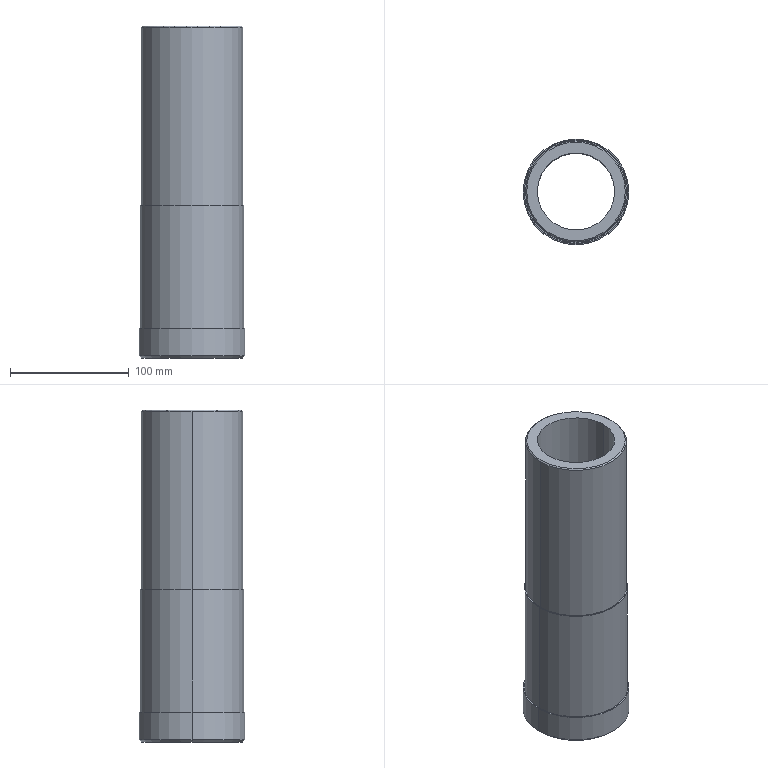Part | SolidWorks | features Chamfer 2, ICE 2, Extrusion 1 | 1 solid | 16 faces | box 89 x 89 x 279.1 mm | volume 698533 mm3 | cylinder 8 | cone 4 | plane 4 | commonest cylinder face diameters 65 x2 85 x2 87 x2 89 x2
STEP:
#1=CARTESIAN_POINT('',(41.5,0.,279.1));
#2=VERTEX_POINT('',#1);
#3=CARTESIAN_POINT('',(-41.5,0.,279.1));
#4=VERTEX_POINT('',#3);
#5=CARTESIAN_POINT('',(0.,0.,279.1));
#6=DIRECTION('',(0.,0.,1.));
#7=DIRECTION('',(1.,0.,0.));
#8=AXIS2_PLACEMENT_3D('',#5,#6,#7);
#9=CIRCLE('',#8,41.5);
#10=EDGE_CURVE('',#2,#4,#9,.T.);
#11=ORIENTED_EDGE('',*,*,#10,.F.);
#12=CARTESIAN_POINT('',(42.5,0.,278.1));
#13=VERTEX_POINT('',#12);
#14=CARTESIAN_POINT('',(41.5,0.,279.1));
#15=DIRECTION('',(0.7071,0.,-0.7071));
#16=VECTOR('',#15,1000.);
#17=LINE('',#14,#16);
#18=EDGE_CURVE('',#2,#13,#17,.T.);
#19=ORIENTED_EDGE('',*,*,#18,.T.);
#20=CARTESIAN_POINT('',(-42.5,0.,278.1));
#21=VERTEX_POINT('',#20);
#22=CARTESIAN_POINT('',(0.,0.,278.1));
#23=DIRECTION('',(0.,0.,-1.));
#24=DIRECTION('',(1.,0.,0.));
#25=AXIS2_PLACEMENT_3D('',#22,#23,#24);
#26=CIRCLE('',#25,42.5);
#27=EDGE_CURVE('',#21,#13,#26,.T.);
#28=ORIENTED_EDGE('',*,*,#27,.F.);
#29=CARTESIAN_POINT('',(-41.5,0.,279.1));
#30=DIRECTION('',(-0.7071,0.,-0.7071));
#31=VECTOR('',#30,1000.);
#32=LINE('',#29,#31);
#33=EDGE_CURVE('',#4,#21,#32,.T.);
#34=ORIENTED_EDGE('',*,*,#33,.F.);
#35=EDGE_LOOP('',(#11,#19,#28,#34));
#36=FACE_OUTER_BOUND('',#35,.T.);
#37=CARTESIAN_POINT('',(0.,0.,279.1));
#38=DIRECTION('',(0.,0.,-1.));
#39=DIRECTION('',(-1.,0.,0.));
#40=AXIS2_PLACEMENT_3D('',#37,#38,#39);
#41=CONICAL_SURFACE('',#40,41.5,0.7854);
#42=ADVANCED_FACE('',(#36),#41,.T.);
#43=CARTESIAN_POINT('',(-42.5,0.,0.));
#44=VERTEX_POINT('',#43);
#45=CARTESIAN_POINT('',(42.5,0.,0.));
#46=VERTEX_POINT('',#45);
#47=CARTESIAN_POINT('',(0.,0.,0.));
#48=DIRECTION('',(0.,0.,-1.));
#49=DIRECTION('',(1.,0.,0.));
#50=AXIS2_PLACEMENT_3D('',#47,#48,#49);
#51=CIRCLE('',#50,42.5);
#52=EDGE_CURVE('',#44,#46,#51,.T.);
#53=ORIENTED_EDGE('',*,*,#52,.F.);
#54=CARTESIAN_POINT('',(-44.5,0.,2.));
#55=VERTEX_POINT('',#54);
#56=CARTESIAN_POINT('',(-44.5,0.,2.));
#57=DIRECTION('',(-0.7071,0.,0.7071));
#58=VECTOR('',#57,1000.);
#59=LINE('',#56,#58);
#60=EDGE_CURVE('',#44,#55,#59,.T.);
#61=ORIENTED_EDGE('',*,*,#60,.T.);
#62=CARTESIAN_POINT('',(44.5,0.,2.));
#63=VERTEX_POINT('',#62);
#64=CARTESIAN_POINT('',(0.,0.,2.));
#65=DIRECTION('',(0.,0.,1.));
#66=DIRECTION('',(1.,0.,0.));
#67=AXIS2_PLACEMENT_3D('',#64,#65,#66);
#68=CIRCLE('',#67,44.5);
#69=EDGE_CURVE('',#63,#55,#68,.T.);
#70=ORIENTED_EDGE('',*,*,#69,.F.);
#71=CARTESIAN_POINT('',(44.5,0.,2.));
#72=DIRECTION('',(0.7071,0.,0.7071));
#73=VECTOR('',#72,1000.);
#74=LINE('',#71,#73);
#75=EDGE_CURVE('',#46,#63,#74,.T.);
#76=ORIENTED_EDGE('',*,*,#75,.F.);
#77=EDGE_LOOP('',(#53,#61,#70,#76));
#78=FACE_OUTER_BOUND('',#77,.T.);
#79=CARTESIAN_POINT('',(0.,0.,2.));
#80=DIRECTION('',(0.,0.,1.));
#81=DIRECTION('',(1.,0.,0.));
#82=AXIS2_PLACEMENT_3D('',#79,#80,#81);
#83=CONICAL_SURFACE('',#82,44.5,0.7854);
#84=ADVANCED_FACE('',(#78),#83,.T.);
#85=CARTESIAN_POINT('',(42.5,0.,128.4));
#86=VERTEX_POINT('',#85);
#87=CARTESIAN_POINT('',(-42.5,0.,128.4));
#88=VERTEX_POINT('',#87);
#89=CARTESIAN_POINT('',(0.,0.,128.4));
#90=DIRECTION('',(0.,0.,1.));
#91=DIRECTION('',(1.,0.,0.));
#92=AXIS2_PLACEMENT_3D('',#89,#90,#91);
#93=CIRCLE('',#92,42.5);
#94=EDGE_CURVE('',#86,#88,#93,.T.);
#95=ORIENTED_EDGE('',*,*,#94,.T.);
#96=CARTESIAN_POINT('',(-42.5,0.,128.4));
#97=DIRECTION('',(0.,0.,1.));
#98=VECTOR('',#97,1000.);
#99=LINE('',#96,#98);
#100=EDGE_CURVE('',#88,#21,#99,.T.);
#101=ORIENTED_EDGE('',*,*,#100,.T.);
#102=ORIENTED_EDGE('',*,*,#27,.T.);
#103=CARTESIAN_POINT('',(42.5,0.,128.4));
#104=DIRECTION('',(0.,0.,1.));
#105=VECTOR('',#104,1000.);
#106=LINE('',#103,#105);
#107=EDGE_CURVE('',#86,#13,#106,.T.);
#108=ORIENTED_EDGE('',*,*,#107,.F.);
#109=EDGE_LOOP('',(#95,#101,#102,#108));
#110=FACE_OUTER_BOUND('',#109,.T.);
#111=CARTESIAN_POINT('',(0.,0.,128.4));
#112=DIRECTION('',(0.,0.,1.));
#113=DIRECTION('',(1.,0.,0.));
#114=AXIS2_PLACEMENT_3D('',#111,#112,#113);
#115=CYLINDRICAL_SURFACE('',#114,42.5);
#116=ADVANCED_FACE('',(#110),#115,.T.);
#117=CARTESIAN_POINT('',(-32.5,0.,279.1));
#118=VERTEX_POINT('',#117);
#119=CARTESIAN_POINT('',(32.5,0.,279.1));
#120=VERTEX_POINT('',#119);
#121=CARTESIAN_POINT('',(0.,0.,279.1));
#122=DIRECTION('',(0.,0.,1.));
#123=DIRECTION('',(1.,0.,0.));
#124=AXIS2_PLACEMENT_3D('',#121,#122,#123);
#125=CIRCLE('',#124,32.5);
#126=EDGE_CURVE('',#118,#120,#125,.T.);
#127=ORIENTED_EDGE('',*,*,#126,.T.);
#128=CARTESIAN_POINT('',(32.5,0.,0.));
#129=VERTEX_POINT('',#128);
#130=CARTESIAN_POINT('',(32.5,0.,279.1));
#131=DIRECTION('',(0.,0.,-1.));
#132=VECTOR('',#131,1000.);
#133=LINE('',#130,#132);
#134=EDGE_CURVE('',#120,#129,#133,.T.);
#135=ORIENTED_EDGE('',*,*,#134,.T.);
#136=CARTESIAN_POINT('',(-32.5,0.,0.));
#137=VERTEX_POINT('',#136);
#138=CARTESIAN_POINT('',(0.,0.,0.));
#139=DIRECTION('',(0.,0.,1.));
#140=DIRECTION('',(1.,0.,0.));
#141=AXIS2_PLACEMENT_3D('',#138,#139,#140);
#142=CIRCLE('',#141,32.5);
#143=EDGE_CURVE('',#137,#129,#142,.T.);
#144=ORIENTED_EDGE('',*,*,#143,.F.);
#145=CARTESIAN_POINT('',(-32.5,0.,279.1));
#146=DIRECTION('',(0.,0.,-1.));
#147=VECTOR('',#146,1000.);
#148=LINE('',#145,#147);
#149=EDGE_CURVE('',#118,#137,#148,.T.);
#150=ORIENTED_EDGE('',*,*,#149,.F.);
#151=EDGE_LOOP('',(#127,#135,#144,#150));
#152=FACE_OUTER_BOUND('',#151,.T.);
#153=CARTESIAN_POINT('',(0.,0.,279.1));
#154=DIRECTION('',(0.,0.,-1.));
#155=DIRECTION('',(-1.,0.,0.));
#156=AXIS2_PLACEMENT_3D('',#153,#154,#155);
#157=CYLINDRICAL_SURFACE('',#156,32.5);
#158=ADVANCED_FACE('',(#152),#157,.F.);
#159=CARTESIAN_POINT('',(-44.5,0.,25.));
#160=VERTEX_POINT('',#159);
#161=CARTESIAN_POINT('',(44.5,0.,25.));
#162=VERTEX_POINT('',#161);
#163=CARTESIAN_POINT('',(0.,0.,25.));
#164=DIRECTION('',(0.,0.,-1.));
#165=DIRECTION('',(-1.,0.,0.));
#166=AXIS2_PLACEMENT_3D('',#163,#164,#165);
#167=CIRCLE('',#166,44.5);
#168=EDGE_CURVE('',#160,#162,#167,.T.);
#169=ORIENTED_EDGE('',*,*,#168,.T.);
#170=CARTESIAN_POINT('',(44.5,0.,279.1));
#171=DIRECTION('',(0.,0.,-1.));
#172=VECTOR('',#171,1000.);
#173=LINE('',#170,#172);
#174=EDGE_CURVE('',#162,#63,#173,.T.);
#175=ORIENTED_EDGE('',*,*,#174,.T.);
#176=ORIENTED_EDGE('',*,*,#69,.T.);
#177=CARTESIAN_POINT('',(-44.5,0.,279.1));
#178=DIRECTION('',(0.,0.,-1.));
#179=VECTOR('',#178,1000.);
#180=LINE('',#177,#179);
#181=EDGE_CURVE('',#160,#55,#180,.T.);
#182=ORIENTED_EDGE('',*,*,#181,.F.);
#183=EDGE_LOOP('',(#169,#175,#176,#182));
#184=FACE_OUTER_BOUND('',#183,.T.);
#185=CARTESIAN_POINT('',(0.,0.,279.1));
#186=DIRECTION('',(0.,0.,-1.));
#187=DIRECTION('',(-1.,0.,0.));
#188=AXIS2_PLACEMENT_3D('',#185,#186,#187);
#189=CYLINDRICAL_SURFACE('',#188,44.5);
#190=ADVANCED_FACE('',(#184),#189,.T.);
#191=CARTESIAN_POINT('',(43.5,0.,128.4));
#192=VERTEX_POINT('',#191);
#193=CARTESIAN_POINT('',(-43.5,0.,128.4));
#194=VERTEX_POINT('',#193);
#195=CARTESIAN_POINT('',(0.,0.,128.4));
#196=DIRECTION('',(0.,0.,1.));
#197=DIRECTION('',(1.,0.,0.));
#198=AXIS2_PLACEMENT_3D('',#195,#196,#197);
#199=CIRCLE('',#198,43.5);
#200=EDGE_CURVE('',#192,#194,#199,.T.);
#201=ORIENTED_EDGE('',*,*,#200,.F.);
#202=CARTESIAN_POINT('',(43.5,0.,25.));
#203=VERTEX_POINT('',#202);
#204=CARTESIAN_POINT('',(43.5,0.,404.965));
#205=DIRECTION('',(0.,0.,-1.));
#206=VECTOR('',#205,1000.);
#207=LINE('',#204,#206);
#208=EDGE_CURVE('',#192,#203,#207,.T.);
#209=ORIENTED_EDGE('',*,*,#208,.T.);
#210=CARTESIAN_POINT('',(-43.5,0.,25.));
#211=VERTEX_POINT('',#210);
#212=CARTESIAN_POINT('',(0.,0.,25.));
#213=DIRECTION('',(0.,0.,-1.));
#214=DIRECTION('',(-1.,0.,0.));
#215=AXIS2_PLACEMENT_3D('',#212,#213,#214);
#216=CIRCLE('',#215,43.5);
#217=EDGE_CURVE('',#211,#203,#216,.T.);
#218=ORIENTED_EDGE('',*,*,#217,.F.);
#219=CARTESIAN_POINT('',(-43.5,0.,404.965));
#220=DIRECTION('',(0.,0.,-1.));
#221=VECTOR('',#220,1000.);
#222=LINE('',#219,#221);
#223=EDGE_CURVE('',#194,#211,#222,.T.);
#224=ORIENTED_EDGE('',*,*,#223,.F.);
#225=EDGE_LOOP('',(#201,#209,#218,#224));
#226=FACE_OUTER_BOUND('',#225,.T.);
#227=CARTESIAN_POINT('',(0.,0.,404.965));
#228=DIRECTION('',(0.,0.,-1.));
#229=DIRECTION('',(-1.,0.,0.));
#230=AXIS2_PLACEMENT_3D('',#227,#228,#229);
#231=CYLINDRICAL_SURFACE('',#230,43.5);
#232=ADVANCED_FACE('',(#226),#231,.T.);
#233=CARTESIAN_POINT('',(0.,0.,279.1));
#234=DIRECTION('',(0.,0.,1.));
#235=DIRECTION('',(1.,0.,0.));
#236=AXIS2_PLACEMENT_3D('',#233,#234,#235);
#237=CIRCLE('',#236,41.5);
#238=EDGE_CURVE('',#4,#2,#237,.T.);
#239=ORIENTED_EDGE('',*,*,#238,.T.);
#240=ORIENTED_EDGE('',*,*,#10,.T.);
#241=EDGE_LOOP('',(#239,#240));
#242=FACE_OUTER_BOUND('',#241,.T.);
#243=ORIENTED_EDGE('',*,*,#126,.F.);
#244=CARTESIAN_POINT('',(0.,0.,279.1));
#245=DIRECTION('',(0.,0.,1.));
#246=DIRECTION('',(1.,0.,0.));
#247=AXIS2_PLACEMENT_3D('',#244,#245,#246);
#248=CIRCLE('',#247,32.5);
#249=EDGE_CURVE('',#120,#118,#248,.T.);
#250=ORIENTED_EDGE('',*,*,#249,.F.);
#251=EDGE_LOOP('',(#243,#250));
#252=FACE_BOUND('',#251,.T.);
#253=CARTESIAN_POINT('',(0.,0.,279.1));
#254=DIRECTION('',(0.,0.,1.));
#255=DIRECTION('',(1.,0.,0.));
#256=AXIS2_PLACEMENT_3D('',#253,#254,#255);
#257=PLANE('',#256);
#258=ADVANCED_FACE('',(#242,#252),#257,.T.);
#259=ORIENTED_EDGE('',*,*,#208,.F.);
#260=CARTESIAN_POINT('',(0.,0.,128.4));
#261=DIRECTION('',(0.,0.,1.));
#262=DIRECTION('',(1.,0.,0.));
#263=AXIS2_PLACEMENT_3D('',#260,#261,#262);
#264=CIRCLE('',#263,43.5);
#265=EDGE_CURVE('',#194,#192,#264,.T.);
#266=ORIENTED_EDGE('',*,*,#265,.F.);
#267=ORIENTED_EDGE('',*,*,#223,.T.);
#268=CARTESIAN_POINT('',(0.,0.,25.));
#269=DIRECTION('',(0.,0.,-1.));
#270=DIRECTION('',(-1.,0.,0.));
#271=AXIS2_PLACEMENT_3D('',#268,#269,#270);
#272=CIRCLE('',#271,43.5);
#273=EDGE_CURVE('',#203,#211,#272,.T.);
#274=ORIENTED_EDGE('',*,*,#273,.F.);
#275=EDGE_LOOP('',(#259,#266,#267,#274));
#276=FACE_OUTER_BOUND('',#275,.T.);
#277=CARTESIAN_POINT('',(0.,0.,404.965));
#278=DIRECTION('',(0.,0.,-1.));
#279=DIRECTION('',(-1.,0.,0.));
#280=AXIS2_PLACEMENT_3D('',#277,#278,#279);
#281=CYLINDRICAL_SURFACE('',#280,43.5);
#282=ADVANCED_FACE('',(#276),#281,.T.);
#283=CARTESIAN_POINT('',(0.,0.,0.));
#284=DIRECTION('',(0.,0.,-1.));
#285=DIRECTION('',(1.,0.,0.));
#286=AXIS2_PLACEMENT_3D('',#283,#284,#285);
#287=CIRCLE('',#286,42.5);
#288=EDGE_CURVE('',#46,#44,#287,.T.);
#289=ORIENTED_EDGE('',*,*,#288,.T.);
#290=ORIENTED_EDGE('',*,*,#52,.T.);
#291=EDGE_LOOP('',(#289,#290));
#292=FACE_OUTER_BOUND('',#291,.T.);
#293=ORIENTED_EDGE('',*,*,#143,.T.);
#294=CARTESIAN_POINT('',(0.,0.,0.));
#295=DIRECTION('',(0.,0.,1.));
#296=DIRECTION('',(1.,0.,0.));
#297=AXIS2_PLACEMENT_3D('',#294,#295,#296);
#298=CIRCLE('',#297,32.5);
#299=EDGE_CURVE('',#129,#137,#298,.T.);
#300=ORIENTED_EDGE('',*,*,#299,.T.);
#301=EDGE_LOOP('',(#293,#300));
#302=FACE_BOUND('',#301,.T.);
#303=CARTESIAN_POINT('',(0.,0.,0.));
#304=DIRECTION('',(0.,0.,1.));
#305=DIRECTION('',(1.,0.,0.));
#306=AXIS2_PLACEMENT_3D('',#303,#304,#305);
#307=PLANE('',#306);
#308=ADVANCED_FACE('',(#292,#302),#307,.F.);
#309=ORIENTED_EDGE('',*,*,#174,.F.);
#310=CARTESIAN_POINT('',(0.,0.,25.));
#311=DIRECTION('',(0.,0.,-1.));
#312=DIRECTION('',(-1.,0.,0.));
#313=AXIS2_PLACEMENT_3D('',#310,#311,#312);
#314=CIRCLE('',#313,44.5);
#315=EDGE_CURVE('',#162,#160,#314,.T.);
#316=ORIENTED_EDGE('',*,*,#315,.T.);
#317=ORIENTED_EDGE('',*,*,#181,.T.);
#318=CARTESIAN_POINT('',(0.,0.,2.));
#319=DIRECTION('',(0.,0.,1.));
#320=DIRECTION('',(1.,0.,0.));
#321=AXIS2_PLACEMENT_3D('',#318,#319,#320);
#322=CIRCLE('',#321,44.5);
#323=EDGE_CURVE('',#55,#63,#322,.T.);
#324=ORIENTED_EDGE('',*,*,#323,.T.);
#325=EDGE_LOOP('',(#309,#316,#317,#324));
#326=FACE_OUTER_BOUND('',#325,.T.);
#327=CARTESIAN_POINT('',(0.,0.,279.1));
#328=DIRECTION('',(0.,0.,-1.));
#329=DIRECTION('',(-1.,0.,0.));
#330=AXIS2_PLACEMENT_3D('',#327,#328,#329);
#331=CYLINDRICAL_SURFACE('',#330,44.5);
#332=ADVANCED_FACE('',(#326),#331,.T.);
#333=ORIENTED_EDGE('',*,*,#134,.F.);
#334=ORIENTED_EDGE('',*,*,#249,.T.);
#335=ORIENTED_EDGE('',*,*,#149,.T.);
#336=ORIENTED_EDGE('',*,*,#299,.F.);
#337=EDGE_LOOP('',(#333,#334,#335,#336));
#338=FACE_OUTER_BOUND('',#337,.T.);
#339=CARTESIAN_POINT('',(0.,0.,279.1));
#340=DIRECTION('',(0.,0.,-1.));
#341=DIRECTION('',(-1.,0.,0.));
#342=AXIS2_PLACEMENT_3D('',#339,#340,#341);
#343=CYLINDRICAL_SURFACE('',#342,32.5);
#344=ADVANCED_FACE('',(#338),#343,.F.);
#345=ORIENTED_EDGE('',*,*,#217,.T.);
#346=ORIENTED_EDGE('',*,*,#273,.T.);
#347=EDGE_LOOP('',(#345,#346));
#348=FACE_BOUND('',#347,.T.);
#349=ORIENTED_EDGE('',*,*,#168,.F.);
#350=ORIENTED_EDGE('',*,*,#315,.F.);
#351=EDGE_LOOP('',(#349,#350));
#352=FACE_OUTER_BOUND('',#351,.T.);
#353=CARTESIAN_POINT('',(0.,0.,25.));
#354=DIRECTION('',(0.,0.,-1.));
#355=DIRECTION('',(-1.,0.,0.));
#356=AXIS2_PLACEMENT_3D('',#353,#354,#355);
#357=PLANE('',#356);
#358=ADVANCED_FACE('',(#348,#352),#357,.F.);
#359=ORIENTED_EDGE('',*,*,#94,.F.);
#360=CARTESIAN_POINT('',(0.,0.,128.4));
#361=DIRECTION('',(0.,0.,1.));
#362=DIRECTION('',(1.,0.,0.));
#363=AXIS2_PLACEMENT_3D('',#360,#361,#362);
#364=CIRCLE('',#363,42.5);
#365=EDGE_CURVE('',#88,#86,#364,.T.);
#366=ORIENTED_EDGE('',*,*,#365,.F.);
#367=EDGE_LOOP('',(#359,#366));
#368=FACE_BOUND('',#367,.T.);
#369=ORIENTED_EDGE('',*,*,#265,.T.);
#370=ORIENTED_EDGE('',*,*,#200,.T.);
#371=EDGE_LOOP('',(#369,#370));
#372=FACE_OUTER_BOUND('',#371,.T.);
#373=CARTESIAN_POINT('',(0.,0.,128.4));
#374=DIRECTION('',(0.,0.,1.));
#375=DIRECTION('',(1.,0.,0.));
#376=AXIS2_PLACEMENT_3D('',#373,#374,#375);
#377=PLANE('',#376);
#378=ADVANCED_FACE('',(#368,#372),#377,.T.);
#379=ORIENTED_EDGE('',*,*,#100,.F.);
#380=ORIENTED_EDGE('',*,*,#365,.T.);
#381=ORIENTED_EDGE('',*,*,#107,.T.);
#382=CARTESIAN_POINT('',(0.,0.,278.1));
#383=DIRECTION('',(0.,0.,-1.));
#384=DIRECTION('',(1.,0.,0.));
#385=AXIS2_PLACEMENT_3D('',#382,#383,#384);
#386=CIRCLE('',#385,42.5);
#387=EDGE_CURVE('',#13,#21,#386,.T.);
#388=ORIENTED_EDGE('',*,*,#387,.T.);
#389=EDGE_LOOP('',(#379,#380,#381,#388));
#390=FACE_OUTER_BOUND('',#389,.T.);
#391=CARTESIAN_POINT('',(0.,0.,128.4));
#392=DIRECTION('',(0.,0.,1.));
#393=DIRECTION('',(1.,0.,0.));
#394=AXIS2_PLACEMENT_3D('',#391,#392,#393);
#395=CYLINDRICAL_SURFACE('',#394,42.5);
#396=ADVANCED_FACE('',(#390),#395,.T.);
#397=ORIENTED_EDGE('',*,*,#60,.F.);
#398=ORIENTED_EDGE('',*,*,#288,.F.);
#399=ORIENTED_EDGE('',*,*,#75,.T.);
#400=ORIENTED_EDGE('',*,*,#323,.F.);
#401=EDGE_LOOP('',(#397,#398,#399,#400));
#402=FACE_OUTER_BOUND('',#401,.T.);
#403=CARTESIAN_POINT('',(0.,0.,2.));
#404=DIRECTION('',(0.,0.,1.));
#405=DIRECTION('',(1.,0.,0.));
#406=AXIS2_PLACEMENT_3D('',#403,#404,#405);
#407=CONICAL_SURFACE('',#406,44.5,0.7854);
#408=ADVANCED_FACE('',(#402),#407,.T.);
#409=ORIENTED_EDGE('',*,*,#18,.F.);
#410=ORIENTED_EDGE('',*,*,#238,.F.);
#411=ORIENTED_EDGE('',*,*,#33,.T.);
#412=ORIENTED_EDGE('',*,*,#387,.F.);
#413=EDGE_LOOP('',(#409,#410,#411,#412));
#414=FACE_OUTER_BOUND('',#413,.T.);
#415=CARTESIAN_POINT('',(0.,0.,279.1));
#416=DIRECTION('',(0.,0.,-1.));
#417=DIRECTION('',(-1.,0.,0.));
#418=AXIS2_PLACEMENT_3D('',#415,#416,#417);
#419=CONICAL_SURFACE('',#418,41.5,0.7854);
#420=ADVANCED_FACE('',(#414),#419,.T.);
#421=CLOSED_SHELL('',(#42,#84,#116,#158,#190,#232,#258,#282,#308,#332,#344,#358,#378,#396,#408,#420));
#422=MANIFOLD_SOLID_BREP('',#421);
#423=CARTESIAN_POINT('',(0.,0.,0.));
#424=DIRECTION('',(0.,0.,1.));
#425=DIRECTION('',(1.,0.,0.));
#426=AXIS2_PLACEMENT_3D('',#423,#424,#425);
#427=(LENGTH_UNIT()NAMED_UNIT(*)SI_UNIT(.MILLI.,.METRE.));
#428=UNCERTAINTY_MEASURE_WITH_UNIT(LENGTH_MEASURE(0.00001),#427,'','');
#429=(NAMED_UNIT(*)PLANE_ANGLE_UNIT()SI_UNIT($,.RADIAN.));
#430=(NAMED_UNIT(*)SI_UNIT($,.STERADIAN.)SOLID_ANGLE_UNIT());
#431=(GEOMETRIC_REPRESENTATION_CONTEXT(3)GLOBAL_UNCERTAINTY_ASSIGNED_CONTEXT((#428))GLOBAL_UNIT_ASSIGNED_CONTEXT((#427,#429,#430))REPRESENTATION_CONTEXT('',''));
#432=ADVANCED_BREP_SHAPE_REPRESENTATION('',(#422,#426),#431);